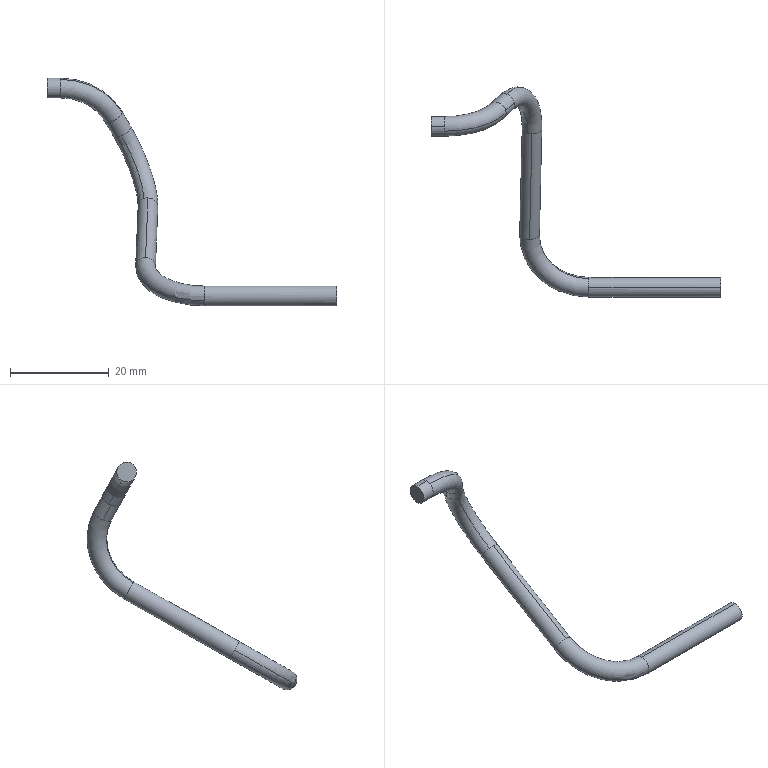Part | SolidWorks | features 3DProfileFeature 2, Sweep 1 | 1 solid | 16 faces | box 58.57 x 42.483 x 46.069 mm | volume 1368 mm3 | cylinder 8 | torus 6 | plane 2 | commonest cylinder face diameters 4 x8
STEP:
#1=CARTESIAN_POINT('',(0.4883,33.183,-32.044));
#2=VERTEX_POINT('',#1);
#3=CARTESIAN_POINT('',(-1.511,34.203,-33.765));
#4=VERTEX_POINT('',#3);
#5=CARTESIAN_POINT('',(0.4883,34.168,-33.785));
#6=DIRECTION('',(-0.02017,-0.8701,-0.4924));
#7=DIRECTION('',(-0.9985,-0.007839,0.05474));
#8=AXIS2_PLACEMENT_3D('',#5,#6,#7);
#9=CIRCLE('',#8,2.);
#10=EDGE_CURVE('',#2,#4,#9,.T.);
#11=ORIENTED_EDGE('',*,*,#10,.T.);
#12=CARTESIAN_POINT('',(12.486,21.773,-40.799));
#13=VERTEX_POINT('',#12);
#14=CARTESIAN_POINT('',(12.486,33.957,-33.904));
#15=DIRECTION('',(0.,-0.4925,0.8703));
#16=DIRECTION('',(0.,-0.8703,-0.4925));
#17=AXIS2_PLACEMENT_3D('',#14,#15,#16);
#18=CIRCLE('',#17,14.);
#19=EDGE_CURVE('',#4,#13,#18,.T.);
#20=ORIENTED_EDGE('',*,*,#19,.T.);
#21=CARTESIAN_POINT('',(12.486,23.514,-37.814));
#22=VERTEX_POINT('',#21);
#23=CARTESIAN_POINT('',(12.486,23.514,-39.814));
#24=DIRECTION('',(1.,0.,0.));
#25=DIRECTION('',(0.,-0.8945,-0.447));
#26=AXIS2_PLACEMENT_3D('',#23,#24,#25);
#27=CIRCLE('',#26,2.);
#28=EDGE_CURVE('',#22,#13,#27,.T.);
#29=ORIENTED_EDGE('',*,*,#28,.F.);
#30=CARTESIAN_POINT('',(12.486,25.254,-38.829));
#31=VERTEX_POINT('',#30);
#32=CARTESIAN_POINT('',(12.486,23.514,-39.814));
#33=DIRECTION('',(1.,0.,0.));
#34=DIRECTION('',(0.,-0.8945,-0.447));
#35=AXIS2_PLACEMENT_3D('',#32,#33,#34);
#36=CIRCLE('',#35,2.);
#37=EDGE_CURVE('',#31,#22,#36,.T.);
#38=ORIENTED_EDGE('',*,*,#37,.F.);
#39=CARTESIAN_POINT('',(2.488,34.133,-33.804));
#40=VERTEX_POINT('',#39);
#41=CARTESIAN_POINT('',(12.486,33.957,-33.904));
#42=DIRECTION('',(0.,-0.4925,0.8703));
#43=DIRECTION('',(0.,-0.8703,-0.4925));
#44=AXIS2_PLACEMENT_3D('',#41,#42,#43);
#45=CIRCLE('',#44,10.);
#46=EDGE_CURVE('',#40,#31,#45,.T.);
#47=ORIENTED_EDGE('',*,*,#46,.F.);
#48=CARTESIAN_POINT('',(0.4883,34.168,-33.785));
#49=DIRECTION('',(-0.02017,-0.8701,-0.4924));
#50=DIRECTION('',(-0.9985,-0.007839,0.05474));
#51=AXIS2_PLACEMENT_3D('',#48,#49,#50);
#52=CIRCLE('',#51,2.);
#53=EDGE_CURVE('',#40,#2,#52,.T.);
#54=ORIENTED_EDGE('',*,*,#53,.T.);
#55=EDGE_LOOP('',(#11,#20,#29,#38,#47,#54));
#56=FACE_OUTER_BOUND('',#55,.T.);
#57=CARTESIAN_POINT('',(12.486,33.957,-33.904));
#58=DIRECTION('',(0.,-0.4925,0.8703));
#59=DIRECTION('',(0.,-0.8703,-0.4925));
#60=AXIS2_PLACEMENT_3D('',#57,#58,#59);
#61=TOROIDAL_SURFACE('',#60,12.,2.);
#62=ADVANCED_FACE('',(#56),#61,.T.);
#63=CARTESIAN_POINT('',(-5.994,60.792,-7.475));
#64=VERTEX_POINT('',#63);
#65=CARTESIAN_POINT('',(-4.23,62.532,-5.476));
#66=VERTEX_POINT('',#65);
#67=CARTESIAN_POINT('',(-4.27,60.792,-6.461));
#68=DIRECTION('',(0.4579,0.4298,-0.7782));
#69=DIRECTION('',(-0.7782,-0.2294,-0.5846));
#70=AXIS2_PLACEMENT_3D('',#67,#68,#69);
#71=CIRCLE('',#70,2.);
#72=EDGE_CURVE('',#64,#66,#71,.T.);
#73=ORIENTED_EDGE('',*,*,#72,.T.);
#74=CARTESIAN_POINT('',(1.899,56.367,-23.265));
#75=VERTEX_POINT('',#74);
#76=CARTESIAN_POINT('',(-4.512,50.351,-12.37));
#77=DIRECTION('',(-0.8888,0.2412,-0.3898));
#78=DIRECTION('',(-0.4016,0.,0.9158));
#79=AXIS2_PLACEMENT_3D('',#76,#77,#78);
#80=CIRCLE('',#79,14.);
#81=EDGE_CURVE('',#66,#75,#80,.T.);
#82=ORIENTED_EDGE('',*,*,#81,.T.);
#83=CARTESIAN_POINT('',(0.9829,56.493,-23.449));
#84=VERTEX_POINT('',#83);
#85=CARTESIAN_POINT('',(0.9829,55.508,-21.708));
#86=DIRECTION('',(-0.02017,-0.8701,-0.4924));
#87=DIRECTION('',(-0.9985,-0.007839,0.05474));
#88=AXIS2_PLACEMENT_3D('',#85,#86,#87);
#89=CIRCLE('',#88,2.);
#90=EDGE_CURVE('',#84,#75,#89,.T.);
#91=ORIENTED_EDGE('',*,*,#90,.F.);
#92=CARTESIAN_POINT('',(0.06709,54.648,-20.152));
#93=VERTEX_POINT('',#92);
#94=CARTESIAN_POINT('',(0.9829,55.508,-21.708));
#95=DIRECTION('',(-0.02017,-0.8701,-0.4924));
#96=DIRECTION('',(-0.9985,-0.007839,0.05474));
#97=AXIS2_PLACEMENT_3D('',#94,#95,#96);
#98=CIRCLE('',#97,2.);
#99=EDGE_CURVE('',#93,#84,#98,.T.);
#100=ORIENTED_EDGE('',*,*,#99,.F.);
#101=CARTESIAN_POINT('',(-4.31,59.052,-7.446));
#102=VERTEX_POINT('',#101);
#103=CARTESIAN_POINT('',(-4.512,50.351,-12.37));
#104=DIRECTION('',(-0.8888,0.2412,-0.3898));
#105=DIRECTION('',(-0.4016,0.,0.9158));
#106=AXIS2_PLACEMENT_3D('',#103,#104,#105);
#107=CIRCLE('',#106,10.);
#108=EDGE_CURVE('',#102,#93,#107,.T.);
#109=ORIENTED_EDGE('',*,*,#108,.F.);
#110=CARTESIAN_POINT('',(-4.27,60.792,-6.461));
#111=DIRECTION('',(0.4579,0.4298,-0.7782));
#112=DIRECTION('',(-0.7782,-0.2294,-0.5846));
#113=AXIS2_PLACEMENT_3D('',#110,#111,#112);
#114=CIRCLE('',#113,2.);
#115=EDGE_CURVE('',#102,#64,#114,.T.);
#116=ORIENTED_EDGE('',*,*,#115,.T.);
#117=EDGE_LOOP('',(#73,#82,#91,#100,#109,#116));
#118=FACE_OUTER_BOUND('',#117,.T.);
#119=CARTESIAN_POINT('',(-4.512,50.351,-12.37));
#120=DIRECTION('',(-0.8888,0.2412,-0.3898));
#121=DIRECTION('',(-0.4016,0.,0.9158));
#122=AXIS2_PLACEMENT_3D('',#119,#120,#121);
#123=TOROIDAL_SURFACE('',#122,12.,2.);
#124=ADVANCED_FACE('',(#118),#123,.T.);
#125=CARTESIAN_POINT('',(-16.716,55.979,4.255));
#126=VERTEX_POINT('',#125);
#127=CARTESIAN_POINT('',(-16.716,55.012,4.006));
#128=VERTEX_POINT('',#127);
#129=CARTESIAN_POINT('',(-16.716,55.979,2.255));
#130=DIRECTION('',(1.,0.,0.));
#131=DIRECTION('',(0.,0.,-1.));
#132=AXIS2_PLACEMENT_3D('',#129,#130,#131);
#133=CIRCLE('',#132,2.);
#134=EDGE_CURVE('',#126,#128,#133,.T.);
#135=ORIENTED_EDGE('',*,*,#134,.T.);
#136=CARTESIAN_POINT('',(-4.27,58.681,-2.638));
#137=VERTEX_POINT('',#136);
#138=CARTESIAN_POINT('',(-16.716,61.78,-8.25));
#139=DIRECTION('',(0.,0.8754,0.4834));
#140=DIRECTION('',(0.,-0.4834,0.8754));
#141=AXIS2_PLACEMENT_3D('',#138,#139,#140);
#142=CIRCLE('',#141,14.);
#143=EDGE_CURVE('',#128,#137,#142,.T.);
#144=ORIENTED_EDGE('',*,*,#143,.T.);
#145=CARTESIAN_POINT('',(-4.324,59.124,-2.425));
#146=VERTEX_POINT('',#145);
#147=CARTESIAN_POINT('',(-6.048,59.124,-3.44));
#148=DIRECTION('',(0.4579,0.4298,-0.7782));
#149=DIRECTION('',(-0.7782,-0.2294,-0.5846));
#150=AXIS2_PLACEMENT_3D('',#147,#148,#149);
#151=CIRCLE('',#150,2.);
#152=EDGE_CURVE('',#146,#137,#151,.T.);
#153=ORIENTED_EDGE('',*,*,#152,.F.);
#154=CARTESIAN_POINT('',(-7.826,59.566,-4.241));
#155=VERTEX_POINT('',#154);
#156=CARTESIAN_POINT('',(-6.048,59.124,-3.44));
#157=DIRECTION('',(0.4579,0.4298,-0.7782));
#158=DIRECTION('',(-0.7782,-0.2294,-0.5846));
#159=AXIS2_PLACEMENT_3D('',#156,#157,#158);
#160=CIRCLE('',#159,2.);
#161=EDGE_CURVE('',#155,#146,#160,.T.);
#162=ORIENTED_EDGE('',*,*,#161,.F.);
#163=CARTESIAN_POINT('',(-16.716,56.946,0.5042));
#164=VERTEX_POINT('',#163);
#165=CARTESIAN_POINT('',(-16.716,61.78,-8.25));
#166=DIRECTION('',(0.,0.8754,0.4834));
#167=DIRECTION('',(0.,-0.4834,0.8754));
#168=AXIS2_PLACEMENT_3D('',#165,#166,#167);
#169=CIRCLE('',#168,10.);
#170=EDGE_CURVE('',#164,#155,#169,.T.);
#171=ORIENTED_EDGE('',*,*,#170,.F.);
#172=CARTESIAN_POINT('',(-16.716,55.979,2.255));
#173=DIRECTION('',(1.,0.,0.));
#174=DIRECTION('',(0.,0.,-1.));
#175=AXIS2_PLACEMENT_3D('',#172,#173,#174);
#176=CIRCLE('',#175,2.);
#177=EDGE_CURVE('',#164,#126,#176,.T.);
#178=ORIENTED_EDGE('',*,*,#177,.T.);
#179=EDGE_LOOP('',(#135,#144,#153,#162,#171,#178));
#180=FACE_OUTER_BOUND('',#179,.T.);
#181=CARTESIAN_POINT('',(-16.716,61.78,-8.25));
#182=DIRECTION('',(0.,0.8754,0.4834));
#183=DIRECTION('',(0.,-0.4834,0.8754));
#184=AXIS2_PLACEMENT_3D('',#181,#182,#183);
#185=TOROIDAL_SURFACE('',#184,12.,2.);
#186=ADVANCED_FACE('',(#180),#185,.T.);
#187=CARTESIAN_POINT('',(12.486,23.514,-41.814));
#188=VERTEX_POINT('',#187);
#189=CARTESIAN_POINT('',(12.486,23.514,-39.814));
#190=DIRECTION('',(1.,0.,0.));
#191=DIRECTION('',(0.,-0.8945,-0.447));
#192=AXIS2_PLACEMENT_3D('',#189,#190,#191);
#193=CIRCLE('',#192,2.);
#194=EDGE_CURVE('',#188,#31,#193,.T.);
#195=ORIENTED_EDGE('',*,*,#194,.T.);
#196=ORIENTED_EDGE('',*,*,#37,.T.);
#197=CARTESIAN_POINT('',(39.172,23.514,-37.814));
#198=VERTEX_POINT('',#197);
#199=CARTESIAN_POINT('',(12.486,23.514,-37.814));
#200=DIRECTION('',(1.,0.,0.));
#201=VECTOR('',#200,1000.);
#202=LINE('',#199,#201);
#203=EDGE_CURVE('',#22,#198,#202,.T.);
#204=ORIENTED_EDGE('',*,*,#203,.T.);
#205=CARTESIAN_POINT('',(39.172,23.514,-41.814));
#206=VERTEX_POINT('',#205);
#207=CARTESIAN_POINT('',(39.172,23.514,-39.814));
#208=DIRECTION('',(1.,0.,0.));
#209=DIRECTION('',(0.,-0.8945,-0.447));
#210=AXIS2_PLACEMENT_3D('',#207,#208,#209);
#211=CIRCLE('',#210,2.);
#212=EDGE_CURVE('',#206,#198,#211,.T.);
#213=ORIENTED_EDGE('',*,*,#212,.F.);
#214=CARTESIAN_POINT('',(12.486,23.514,-41.814));
#215=DIRECTION('',(1.,0.,0.));
#216=VECTOR('',#215,1000.);
#217=LINE('',#214,#216);
#218=EDGE_CURVE('',#188,#206,#217,.T.);
#219=ORIENTED_EDGE('',*,*,#218,.F.);
#220=EDGE_LOOP('',(#195,#196,#204,#213,#219));
#221=FACE_OUTER_BOUND('',#220,.T.);
#222=CARTESIAN_POINT('',(12.486,23.514,-39.814));
#223=DIRECTION('',(1.,0.,0.));
#224=DIRECTION('',(0.,0.,-1.));
#225=AXIS2_PLACEMENT_3D('',#222,#223,#224);
#226=CYLINDRICAL_SURFACE('',#225,2.);
#227=ADVANCED_FACE('',(#221),#226,.T.);
#228=ORIENTED_EDGE('',*,*,#90,.T.);
#229=CARTESIAN_POINT('',(0.9829,54.523,-19.968));
#230=VERTEX_POINT('',#229);
#231=CARTESIAN_POINT('',(0.9829,55.508,-21.708));
#232=DIRECTION('',(-0.02017,-0.8701,-0.4924));
#233=DIRECTION('',(-0.9985,-0.007839,0.05474));
#234=AXIS2_PLACEMENT_3D('',#231,#232,#233);
#235=CIRCLE('',#234,2.);
#236=EDGE_CURVE('',#75,#230,#235,.T.);
#237=ORIENTED_EDGE('',*,*,#236,.T.);
#238=CARTESIAN_POINT('',(0.9829,54.523,-19.968));
#239=DIRECTION('',(-0.02017,-0.8701,-0.4924));
#240=VECTOR('',#239,1000.);
#241=LINE('',#238,#240);
#242=EDGE_CURVE('',#230,#2,#241,.T.);
#243=ORIENTED_EDGE('',*,*,#242,.T.);
#244=ORIENTED_EDGE('',*,*,#53,.F.);
#245=CARTESIAN_POINT('',(0.4883,35.153,-35.525));
#246=VERTEX_POINT('',#245);
#247=CARTESIAN_POINT('',(0.4883,34.168,-33.785));
#248=DIRECTION('',(-0.02017,-0.8701,-0.4924));
#249=DIRECTION('',(-0.9985,-0.007839,0.05474));
#250=AXIS2_PLACEMENT_3D('',#247,#248,#249);
#251=CIRCLE('',#250,2.);
#252=EDGE_CURVE('',#246,#40,#251,.T.);
#253=ORIENTED_EDGE('',*,*,#252,.F.);
#254=CARTESIAN_POINT('',(0.9829,56.493,-23.449));
#255=DIRECTION('',(-0.02017,-0.8701,-0.4924));
#256=VECTOR('',#255,1000.);
#257=LINE('',#254,#256);
#258=EDGE_CURVE('',#84,#246,#257,.T.);
#259=ORIENTED_EDGE('',*,*,#258,.F.);
#260=EDGE_LOOP('',(#228,#237,#243,#244,#253,#259));
#261=FACE_OUTER_BOUND('',#260,.T.);
#262=CARTESIAN_POINT('',(0.9829,55.508,-21.708));
#263=DIRECTION('',(-0.02017,-0.8701,-0.4924));
#264=DIRECTION('',(0.,0.4925,-0.8703));
#265=AXIS2_PLACEMENT_3D('',#262,#263,#264);
#266=CYLINDRICAL_SURFACE('',#265,2.);
#267=ADVANCED_FACE('',(#261),#266,.T.);
#268=CARTESIAN_POINT('',(-7.771,59.124,-4.454));
#269=VERTEX_POINT('',#268);
#270=CARTESIAN_POINT('',(-6.048,59.124,-3.44));
#271=DIRECTION('',(0.4579,0.4298,-0.7782));
#272=DIRECTION('',(-0.7782,-0.2294,-0.5846));
#273=AXIS2_PLACEMENT_3D('',#270,#271,#272);
#274=CIRCLE('',#273,2.);
#275=EDGE_CURVE('',#269,#155,#274,.T.);
#276=ORIENTED_EDGE('',*,*,#275,.T.);
#277=ORIENTED_EDGE('',*,*,#161,.T.);
#278=CARTESIAN_POINT('',(-2.546,60.792,-5.447));
#279=VERTEX_POINT('',#278);
#280=CARTESIAN_POINT('',(-4.324,59.124,-2.425));
#281=DIRECTION('',(0.4579,0.4298,-0.7782));
#282=VECTOR('',#281,1000.);
#283=LINE('',#280,#282);
#284=EDGE_CURVE('',#146,#279,#283,.T.);
#285=ORIENTED_EDGE('',*,*,#284,.T.);
#286=CARTESIAN_POINT('',(-4.27,60.792,-6.461));
#287=DIRECTION('',(0.4579,0.4298,-0.7782));
#288=DIRECTION('',(-0.7782,-0.2294,-0.5846));
#289=AXIS2_PLACEMENT_3D('',#286,#287,#288);
#290=CIRCLE('',#289,2.);
#291=EDGE_CURVE('',#66,#279,#290,.T.);
#292=ORIENTED_EDGE('',*,*,#291,.F.);
#293=ORIENTED_EDGE('',*,*,#72,.F.);
#294=CARTESIAN_POINT('',(-7.771,59.124,-4.454));
#295=DIRECTION('',(0.4579,0.4298,-0.7782));
#296=VECTOR('',#295,1000.);
#297=LINE('',#294,#296);
#298=EDGE_CURVE('',#269,#64,#297,.T.);
#299=ORIENTED_EDGE('',*,*,#298,.F.);
#300=EDGE_LOOP('',(#276,#277,#285,#292,#293,#299));
#301=FACE_OUTER_BOUND('',#300,.T.);
#302=CARTESIAN_POINT('',(-6.048,59.124,-3.44));
#303=DIRECTION('',(0.4579,0.4298,-0.7782));
#304=DIRECTION('',(-0.8619,0.,-0.5071));
#305=AXIS2_PLACEMENT_3D('',#302,#303,#304);
#306=CYLINDRICAL_SURFACE('',#305,2.);
#307=ADVANCED_FACE('',(#301),#306,.T.);
#308=CARTESIAN_POINT('',(-19.398,55.979,0.2549));
#309=VERTEX_POINT('',#308);
#310=CARTESIAN_POINT('',(-19.398,55.979,4.255));
#311=VERTEX_POINT('',#310);
#312=CARTESIAN_POINT('',(-19.398,55.979,2.255));
#313=DIRECTION('',(1.,0.,0.));
#314=DIRECTION('',(0.,0.,-1.));
#315=AXIS2_PLACEMENT_3D('',#312,#313,#314);
#316=CIRCLE('',#315,2.);
#317=EDGE_CURVE('',#309,#311,#316,.T.);
#318=ORIENTED_EDGE('',*,*,#317,.T.);
#319=CARTESIAN_POINT('',(-19.398,55.979,4.255));
#320=DIRECTION('',(1.,0.,0.));
#321=VECTOR('',#320,1000.);
#322=LINE('',#319,#321);
#323=EDGE_CURVE('',#311,#126,#322,.T.);
#324=ORIENTED_EDGE('',*,*,#323,.T.);
#325=ORIENTED_EDGE('',*,*,#177,.F.);
#326=CARTESIAN_POINT('',(-16.716,55.979,0.2549));
#327=VERTEX_POINT('',#326);
#328=CARTESIAN_POINT('',(-16.716,55.979,2.255));
#329=DIRECTION('',(1.,0.,0.));
#330=DIRECTION('',(0.,0.,-1.));
#331=AXIS2_PLACEMENT_3D('',#328,#329,#330);
#332=CIRCLE('',#331,2.);
#333=EDGE_CURVE('',#327,#164,#332,.T.);
#334=ORIENTED_EDGE('',*,*,#333,.F.);
#335=CARTESIAN_POINT('',(-19.398,55.979,0.2549));
#336=DIRECTION('',(1.,0.,0.));
#337=VECTOR('',#336,1000.);
#338=LINE('',#335,#337);
#339=EDGE_CURVE('',#309,#327,#338,.T.);
#340=ORIENTED_EDGE('',*,*,#339,.F.);
#341=EDGE_LOOP('',(#318,#324,#325,#334,#340));
#342=FACE_OUTER_BOUND('',#341,.T.);
#343=CARTESIAN_POINT('',(-19.398,55.979,2.255));
#344=DIRECTION('',(1.,0.,0.));
#345=DIRECTION('',(0.,0.,-1.));
#346=AXIS2_PLACEMENT_3D('',#343,#344,#345);
#347=CYLINDRICAL_SURFACE('',#346,2.);
#348=ADVANCED_FACE('',(#342),#347,.T.);
#349=ORIENTED_EDGE('',*,*,#203,.F.);
#350=ORIENTED_EDGE('',*,*,#28,.T.);
#351=CARTESIAN_POINT('',(12.486,23.514,-39.814));
#352=DIRECTION('',(1.,0.,0.));
#353=DIRECTION('',(0.,-0.8945,-0.447));
#354=AXIS2_PLACEMENT_3D('',#351,#352,#353);
#355=CIRCLE('',#354,2.);
#356=EDGE_CURVE('',#13,#188,#355,.T.);
#357=ORIENTED_EDGE('',*,*,#356,.T.);
#358=ORIENTED_EDGE('',*,*,#218,.T.);
#359=CARTESIAN_POINT('',(39.172,23.514,-39.814));
#360=DIRECTION('',(1.,0.,0.));
#361=DIRECTION('',(0.,-0.8945,-0.447));
#362=AXIS2_PLACEMENT_3D('',#359,#360,#361);
#363=CIRCLE('',#362,2.);
#364=EDGE_CURVE('',#198,#206,#363,.T.);
#365=ORIENTED_EDGE('',*,*,#364,.F.);
#366=EDGE_LOOP('',(#349,#350,#357,#358,#365));
#367=FACE_OUTER_BOUND('',#366,.T.);
#368=CARTESIAN_POINT('',(12.486,23.514,-39.814));
#369=DIRECTION('',(1.,0.,0.));
#370=DIRECTION('',(0.,0.,-1.));
#371=AXIS2_PLACEMENT_3D('',#368,#369,#370);
#372=CYLINDRICAL_SURFACE('',#371,2.);
#373=ADVANCED_FACE('',(#367),#372,.T.);
#374=ORIENTED_EDGE('',*,*,#19,.F.);
#375=CARTESIAN_POINT('',(0.4883,34.168,-33.785));
#376=DIRECTION('',(-0.02017,-0.8701,-0.4924));
#377=DIRECTION('',(-0.9985,-0.007839,0.05474));
#378=AXIS2_PLACEMENT_3D('',#375,#376,#377);
#379=CIRCLE('',#378,2.);
#380=EDGE_CURVE('',#4,#246,#379,.T.);
#381=ORIENTED_EDGE('',*,*,#380,.T.);
#382=ORIENTED_EDGE('',*,*,#252,.T.);
#383=ORIENTED_EDGE('',*,*,#46,.T.);
#384=ORIENTED_EDGE('',*,*,#194,.F.);
#385=ORIENTED_EDGE('',*,*,#356,.F.);
#386=EDGE_LOOP('',(#374,#381,#382,#383,#384,#385));
#387=FACE_OUTER_BOUND('',#386,.T.);
#388=CARTESIAN_POINT('',(12.486,33.957,-33.904));
#389=DIRECTION('',(0.,-0.4925,0.8703));
#390=DIRECTION('',(0.,-0.8703,-0.4925));
#391=AXIS2_PLACEMENT_3D('',#388,#389,#390);
#392=TOROIDAL_SURFACE('',#391,12.,2.);
#393=ADVANCED_FACE('',(#387),#392,.T.);
#394=ORIENTED_EDGE('',*,*,#242,.F.);
#395=CARTESIAN_POINT('',(0.9829,55.508,-21.708));
#396=DIRECTION('',(-0.02017,-0.8701,-0.4924));
#397=DIRECTION('',(-0.9985,-0.007839,0.05474));
#398=AXIS2_PLACEMENT_3D('',#395,#396,#397);
#399=CIRCLE('',#398,2.);
#400=EDGE_CURVE('',#230,#93,#399,.T.);
#401=ORIENTED_EDGE('',*,*,#400,.T.);
#402=ORIENTED_EDGE('',*,*,#99,.T.);
#403=ORIENTED_EDGE('',*,*,#258,.T.);
#404=ORIENTED_EDGE('',*,*,#380,.F.);
#405=ORIENTED_EDGE('',*,*,#10,.F.);
#406=EDGE_LOOP('',(#394,#401,#402,#403,#404,#405));
#407=FACE_OUTER_BOUND('',#406,.T.);
#408=CARTESIAN_POINT('',(0.9829,55.508,-21.708));
#409=DIRECTION('',(-0.02017,-0.8701,-0.4924));
#410=DIRECTION('',(0.,0.4925,-0.8703));
#411=AXIS2_PLACEMENT_3D('',#408,#409,#410);
#412=CYLINDRICAL_SURFACE('',#411,2.);
#413=ADVANCED_FACE('',(#407),#412,.T.);
#414=ORIENTED_EDGE('',*,*,#81,.F.);
#415=ORIENTED_EDGE('',*,*,#291,.T.);
#416=CARTESIAN_POINT('',(-4.27,60.792,-6.461));
#417=DIRECTION('',(0.4579,0.4298,-0.7782));
#418=DIRECTION('',(-0.7782,-0.2294,-0.5846));
#419=AXIS2_PLACEMENT_3D('',#416,#417,#418);
#420=CIRCLE('',#419,2.);
#421=EDGE_CURVE('',#279,#102,#420,.T.);
#422=ORIENTED_EDGE('',*,*,#421,.T.);
#423=ORIENTED_EDGE('',*,*,#108,.T.);
#424=ORIENTED_EDGE('',*,*,#400,.F.);
#425=ORIENTED_EDGE('',*,*,#236,.F.);
#426=EDGE_LOOP('',(#414,#415,#422,#423,#424,#425));
#427=FACE_OUTER_BOUND('',#426,.T.);
#428=CARTESIAN_POINT('',(-4.512,50.351,-12.37));
#429=DIRECTION('',(-0.8888,0.2412,-0.3898));
#430=DIRECTION('',(-0.4016,0.,0.9158));
#431=AXIS2_PLACEMENT_3D('',#428,#429,#430);
#432=TOROIDAL_SURFACE('',#431,12.,2.);
#433=ADVANCED_FACE('',(#427),#432,.T.);
#434=ORIENTED_EDGE('',*,*,#284,.F.);
#435=ORIENTED_EDGE('',*,*,#152,.T.);
#436=CARTESIAN_POINT('',(-6.048,59.124,-3.44));
#437=DIRECTION('',(0.4579,0.4298,-0.7782));
#438=DIRECTION('',(-0.7782,-0.2294,-0.5846));
#439=AXIS2_PLACEMENT_3D('',#436,#437,#438);
#440=CIRCLE('',#439,2.);
#441=EDGE_CURVE('',#137,#269,#440,.T.);
#442=ORIENTED_EDGE('',*,*,#441,.T.);
#443=ORIENTED_EDGE('',*,*,#298,.T.);
#444=ORIENTED_EDGE('',*,*,#115,.F.);
#445=ORIENTED_EDGE('',*,*,#421,.F.);
#446=EDGE_LOOP('',(#434,#435,#442,#443,#444,#445));
#447=FACE_OUTER_BOUND('',#446,.T.);
#448=CARTESIAN_POINT('',(-6.048,59.124,-3.44));
#449=DIRECTION('',(0.4579,0.4298,-0.7782));
#450=DIRECTION('',(-0.8619,0.,-0.5071));
#451=AXIS2_PLACEMENT_3D('',#448,#449,#450);
#452=CYLINDRICAL_SURFACE('',#451,2.);
#453=ADVANCED_FACE('',(#447),#452,.T.);
#454=ORIENTED_EDGE('',*,*,#143,.F.);
#455=CARTESIAN_POINT('',(-16.716,55.979,2.255));
#456=DIRECTION('',(1.,0.,0.));
#457=DIRECTION('',(0.,0.,-1.));
#458=AXIS2_PLACEMENT_3D('',#455,#456,#457);
#459=CIRCLE('',#458,2.);
#460=EDGE_CURVE('',#128,#327,#459,.T.);
#461=ORIENTED_EDGE('',*,*,#460,.T.);
#462=ORIENTED_EDGE('',*,*,#333,.T.);
#463=ORIENTED_EDGE('',*,*,#170,.T.);
#464=ORIENTED_EDGE('',*,*,#275,.F.);
#465=ORIENTED_EDGE('',*,*,#441,.F.);
#466=EDGE_LOOP('',(#454,#461,#462,#463,#464,#465));
#467=FACE_OUTER_BOUND('',#466,.T.);
#468=CARTESIAN_POINT('',(-16.716,61.78,-8.25));
#469=DIRECTION('',(0.,0.8754,0.4834));
#470=DIRECTION('',(0.,-0.4834,0.8754));
#471=AXIS2_PLACEMENT_3D('',#468,#469,#470);
#472=TOROIDAL_SURFACE('',#471,12.,2.);
#473=ADVANCED_FACE('',(#467),#472,.T.);
#474=ORIENTED_EDGE('',*,*,#323,.F.);
#475=CARTESIAN_POINT('',(-19.398,55.979,2.255));
#476=DIRECTION('',(1.,0.,0.));
#477=DIRECTION('',(0.,0.,-1.));
#478=AXIS2_PLACEMENT_3D('',#475,#476,#477);
#479=CIRCLE('',#478,2.);
#480=EDGE_CURVE('',#311,#309,#479,.T.);
#481=ORIENTED_EDGE('',*,*,#480,.T.);
#482=ORIENTED_EDGE('',*,*,#339,.T.);
#483=ORIENTED_EDGE('',*,*,#460,.F.);
#484=ORIENTED_EDGE('',*,*,#134,.F.);
#485=EDGE_LOOP('',(#474,#481,#482,#483,#484));
#486=FACE_OUTER_BOUND('',#485,.T.);
#487=CARTESIAN_POINT('',(-19.398,55.979,2.255));
#488=DIRECTION('',(1.,0.,0.));
#489=DIRECTION('',(0.,0.,-1.));
#490=AXIS2_PLACEMENT_3D('',#487,#488,#489);
#491=CYLINDRICAL_SURFACE('',#490,2.);
#492=ADVANCED_FACE('',(#486),#491,.T.);
#493=ORIENTED_EDGE('',*,*,#212,.T.);
#494=ORIENTED_EDGE('',*,*,#364,.T.);
#495=EDGE_LOOP('',(#493,#494));
#496=FACE_OUTER_BOUND('',#495,.T.);
#497=CARTESIAN_POINT('',(39.172,23.514,-39.814));
#498=DIRECTION('',(1.,0.,0.));
#499=DIRECTION('',(0.,-0.8945,-0.447));
#500=AXIS2_PLACEMENT_3D('',#497,#498,#499);
#501=PLANE('',#500);
#502=ADVANCED_FACE('',(#496),#501,.T.);
#503=ORIENTED_EDGE('',*,*,#317,.F.);
#504=ORIENTED_EDGE('',*,*,#480,.F.);
#505=EDGE_LOOP('',(#503,#504));
#506=FACE_OUTER_BOUND('',#505,.T.);
#507=CARTESIAN_POINT('',(-19.398,55.979,2.255));
#508=DIRECTION('',(1.,0.,0.));
#509=DIRECTION('',(0.,0.,-1.));
#510=AXIS2_PLACEMENT_3D('',#507,#508,#509);
#511=PLANE('',#510);
#512=ADVANCED_FACE('',(#506),#511,.F.);
#513=CLOSED_SHELL('',(#62,#124,#186,#227,#267,#307,#348,#373,#393,#413,#433,#453,#473,#492,#502,#512));
#514=MANIFOLD_SOLID_BREP('',#513);
#515=CARTESIAN_POINT('',(0.,0.,0.));
#516=DIRECTION('',(0.,0.,1.));
#517=DIRECTION('',(1.,0.,0.));
#518=AXIS2_PLACEMENT_3D('',#515,#516,#517);
#519=(LENGTH_UNIT()NAMED_UNIT(*)SI_UNIT(.MILLI.,.METRE.));
#520=UNCERTAINTY_MEASURE_WITH_UNIT(LENGTH_MEASURE(0.00001),#519,'','');
#521=(NAMED_UNIT(*)PLANE_ANGLE_UNIT()SI_UNIT($,.RADIAN.));
#522=(NAMED_UNIT(*)SI_UNIT($,.STERADIAN.)SOLID_ANGLE_UNIT());
#523=(GEOMETRIC_REPRESENTATION_CONTEXT(3)GLOBAL_UNCERTAINTY_ASSIGNED_CONTEXT((#520))GLOBAL_UNIT_ASSIGNED_CONTEXT((#519,#521,#522))REPRESENTATION_CONTEXT('',''));
#524=ADVANCED_BREP_SHAPE_REPRESENTATION('',(#514,#518),#523);